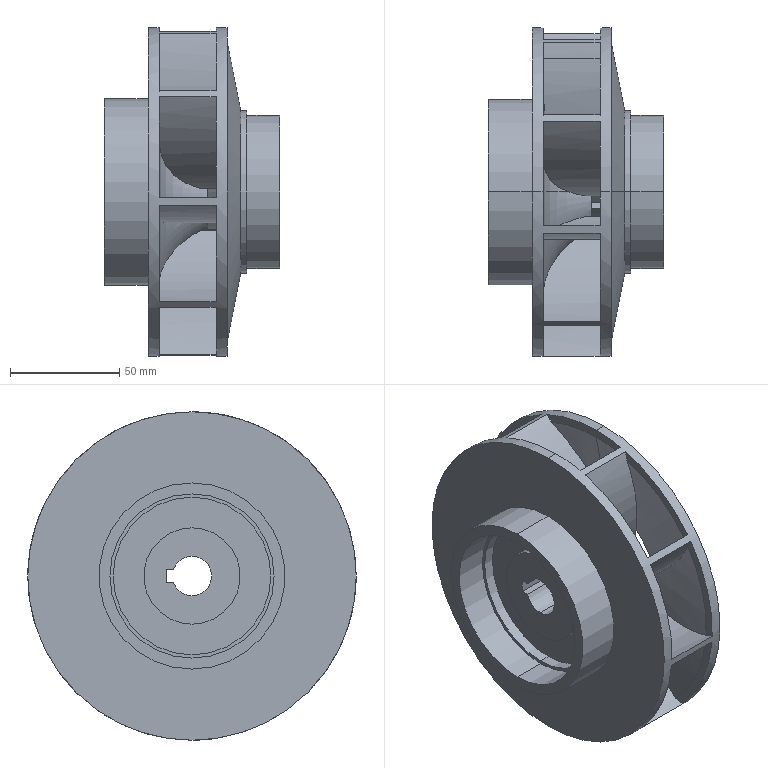Part | SolidWorks | features ICE 3, CirPattern 1, Fillet 1, Revolution 1 | 1 solid | 113 faces | box 80 x 150 x 150 mm | volume 302851 mm3 | cylinder 49 | plane 30 | cone 21 | torus 13 | commonest cylinder face diameters 38 x10 170 x10 176 x10 18 x3 44 x2 60 x2